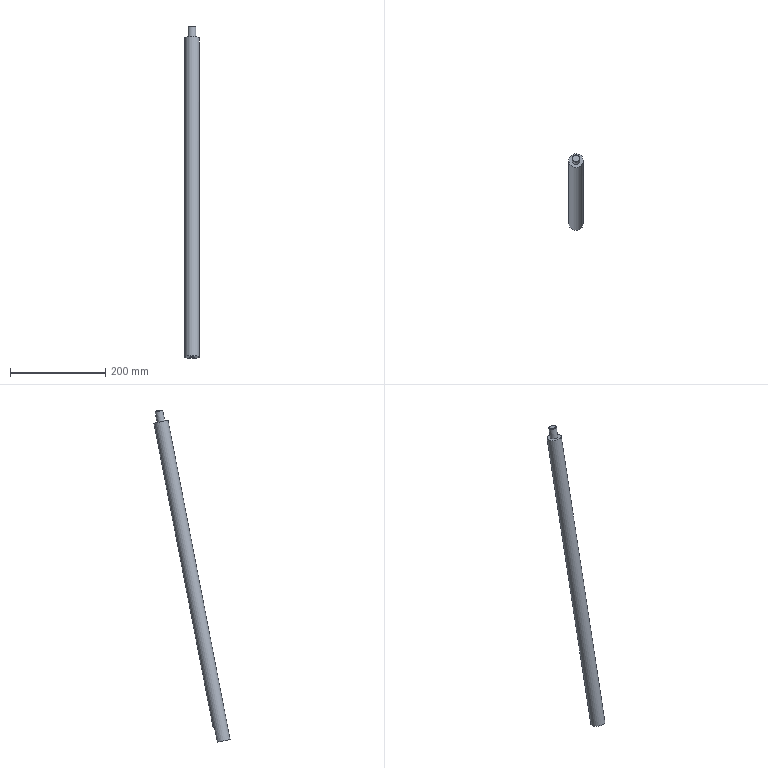Part | STEP file | solid 92 | 1 solid | 11 faces | box 30 x 159.47 x 696.084 mm | volume 483606 mm3 | plane 5 | cylinder 3 | cone 3 | commonest cylinder face diameters 10.2 x1 16 x1 30 x1